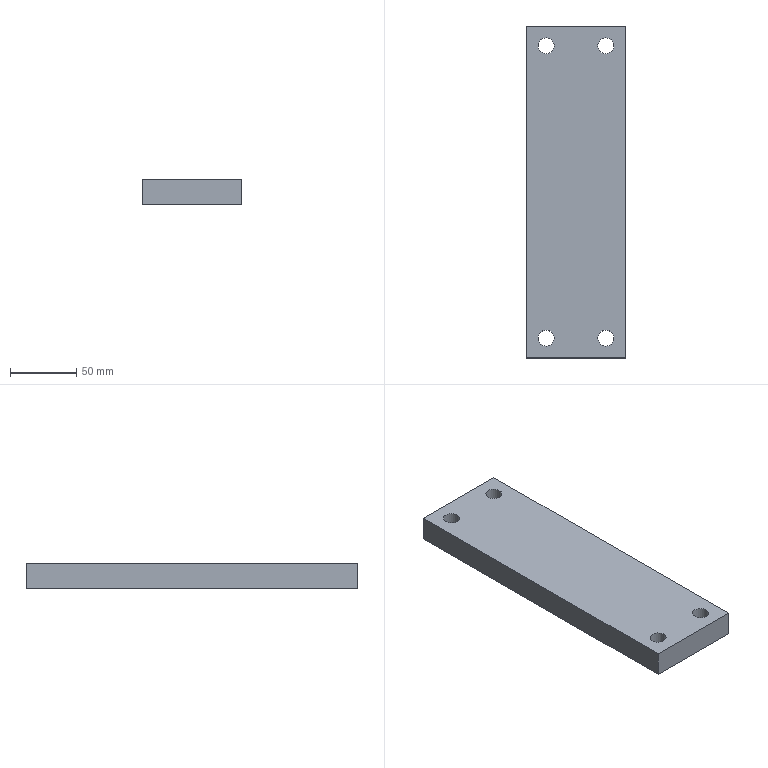Part | NX | features solid 2 | 1 solid | 10 faces | box 75 x 250 x 19 mm | volume 347655 mm3 | plane 6 | cylinder 4 | commonest cylinder face diameters 12 x4
STEP:
#1=CARTESIAN_POINT('',(277.5,-114.,-15.));
#2=VERTEX_POINT('',#1);
#3=CARTESIAN_POINT('',(277.5,-120.,-15.));
#4=DIRECTION('',(0.,0.,1.));
#5=DIRECTION('',(0.,1.,0.));
#6=AXIS2_PLACEMENT_3D('',#3,#4,#5);
#7=CIRCLE('',#6,6.);
#8=EDGE_CURVE('',#2,#2,#7,.T.);
#9=ORIENTED_EDGE('',*,*,#8,.F.);
#10=EDGE_LOOP('',(#9));
#11=FACE_BOUND('',#10,.T.);
#12=CARTESIAN_POINT('',(277.5,106.,-15.));
#13=VERTEX_POINT('',#12);
#14=CARTESIAN_POINT('',(277.5,100.,-15.));
#15=DIRECTION('',(0.,0.,1.));
#16=DIRECTION('',(0.,1.,0.));
#17=AXIS2_PLACEMENT_3D('',#14,#15,#16);
#18=CIRCLE('',#17,6.);
#19=EDGE_CURVE('',#13,#13,#18,.F.);
#20=ORIENTED_EDGE('',*,*,#19,.T.);
#21=EDGE_LOOP('',(#20));
#22=FACE_BOUND('',#21,.T.);
#23=CARTESIAN_POINT('',(232.5,106.,-15.));
#24=VERTEX_POINT('',#23);
#25=CARTESIAN_POINT('',(232.5,100.,-15.));
#26=DIRECTION('',(0.,0.,1.));
#27=DIRECTION('',(0.,1.,0.));
#28=AXIS2_PLACEMENT_3D('',#25,#26,#27);
#29=CIRCLE('',#28,6.);
#30=EDGE_CURVE('',#24,#24,#29,.T.);
#31=ORIENTED_EDGE('',*,*,#30,.F.);
#32=EDGE_LOOP('',(#31));
#33=FACE_BOUND('',#32,.T.);
#34=CARTESIAN_POINT('',(292.5,115.,-15.));
#35=VERTEX_POINT('',#34);
#36=CARTESIAN_POINT('',(292.5,-135.,-15.));
#37=VERTEX_POINT('',#36);
#38=CARTESIAN_POINT('',(292.5,115.,-15.));
#39=DIRECTION('',(0.,-1.,0.));
#40=VECTOR('',#39,1000.);
#41=LINE('',#38,#40);
#42=EDGE_CURVE('',#35,#37,#41,.T.);
#43=ORIENTED_EDGE('',*,*,#42,.F.);
#44=CARTESIAN_POINT('',(217.5,115.,-15.));
#45=VERTEX_POINT('',#44);
#46=CARTESIAN_POINT('',(217.5,115.,-15.));
#47=DIRECTION('',(1.,0.,0.));
#48=VECTOR('',#47,1000.);
#49=LINE('',#46,#48);
#50=EDGE_CURVE('',#45,#35,#49,.T.);
#51=ORIENTED_EDGE('',*,*,#50,.F.);
#52=CARTESIAN_POINT('',(217.5,-135.,-15.));
#53=VERTEX_POINT('',#52);
#54=CARTESIAN_POINT('',(217.5,-135.,-15.));
#55=DIRECTION('',(0.,1.,0.));
#56=VECTOR('',#55,1000.);
#57=LINE('',#54,#56);
#58=EDGE_CURVE('',#53,#45,#57,.T.);
#59=ORIENTED_EDGE('',*,*,#58,.F.);
#60=CARTESIAN_POINT('',(292.5,-135.,-15.));
#61=DIRECTION('',(-1.,0.,0.));
#62=VECTOR('',#61,1000.);
#63=LINE('',#60,#62);
#64=EDGE_CURVE('',#37,#53,#63,.T.);
#65=ORIENTED_EDGE('',*,*,#64,.F.);
#66=EDGE_LOOP('',(#43,#51,#59,#65));
#67=FACE_BOUND('',#66,.T.);
#68=CARTESIAN_POINT('',(232.5,-114.,-15.));
#69=VERTEX_POINT('',#68);
#70=CARTESIAN_POINT('',(232.5,-120.,-15.));
#71=DIRECTION('',(0.,0.,1.));
#72=DIRECTION('',(0.,1.,0.));
#73=AXIS2_PLACEMENT_3D('',#70,#71,#72);
#74=CIRCLE('',#73,6.);
#75=EDGE_CURVE('',#69,#69,#74,.F.);
#76=ORIENTED_EDGE('',*,*,#75,.T.);
#77=EDGE_LOOP('',(#76));
#78=FACE_BOUND('',#77,.T.);
#79=CARTESIAN_POINT('',(292.5,115.,-15.));
#80=DIRECTION('',(0.,0.,1.));
#81=DIRECTION('',(0.,1.,0.));
#82=AXIS2_PLACEMENT_3D('',#79,#80,#81);
#83=PLANE('',#82);
#84=ADVANCED_FACE('',(#11,#22,#33,#67,#78),#83,.T.);
#85=CARTESIAN_POINT('',(277.5,-114.,-34.));
#86=VERTEX_POINT('',#85);
#87=CARTESIAN_POINT('',(277.5,-120.,-34.));
#88=DIRECTION('',(0.,0.,1.));
#89=DIRECTION('',(0.,1.,0.));
#90=AXIS2_PLACEMENT_3D('',#87,#88,#89);
#91=CIRCLE('',#90,6.);
#92=EDGE_CURVE('',#86,#86,#91,.T.);
#93=ORIENTED_EDGE('',*,*,#92,.T.);
#94=EDGE_LOOP('',(#93));
#95=FACE_BOUND('',#94,.T.);
#96=CARTESIAN_POINT('',(277.5,106.,-34.));
#97=VERTEX_POINT('',#96);
#98=CARTESIAN_POINT('',(277.5,100.,-34.));
#99=DIRECTION('',(0.,0.,1.));
#100=DIRECTION('',(0.,1.,0.));
#101=AXIS2_PLACEMENT_3D('',#98,#99,#100);
#102=CIRCLE('',#101,6.);
#103=EDGE_CURVE('',#97,#97,#102,.F.);
#104=ORIENTED_EDGE('',*,*,#103,.F.);
#105=EDGE_LOOP('',(#104));
#106=FACE_BOUND('',#105,.T.);
#107=CARTESIAN_POINT('',(232.5,106.,-34.));
#108=VERTEX_POINT('',#107);
#109=CARTESIAN_POINT('',(232.5,100.,-34.));
#110=DIRECTION('',(0.,0.,1.));
#111=DIRECTION('',(0.,1.,0.));
#112=AXIS2_PLACEMENT_3D('',#109,#110,#111);
#113=CIRCLE('',#112,6.);
#114=EDGE_CURVE('',#108,#108,#113,.T.);
#115=ORIENTED_EDGE('',*,*,#114,.T.);
#116=EDGE_LOOP('',(#115));
#117=FACE_BOUND('',#116,.T.);
#118=CARTESIAN_POINT('',(292.5,115.,-34.));
#119=VERTEX_POINT('',#118);
#120=CARTESIAN_POINT('',(292.5,-135.,-34.));
#121=VERTEX_POINT('',#120);
#122=CARTESIAN_POINT('',(292.5,115.,-34.));
#123=DIRECTION('',(0.,-1.,0.));
#124=VECTOR('',#123,1000.);
#125=LINE('',#122,#124);
#126=EDGE_CURVE('',#119,#121,#125,.T.);
#127=ORIENTED_EDGE('',*,*,#126,.T.);
#128=CARTESIAN_POINT('',(217.5,-135.,-34.));
#129=VERTEX_POINT('',#128);
#130=CARTESIAN_POINT('',(292.5,-135.,-34.));
#131=DIRECTION('',(-1.,0.,0.));
#132=VECTOR('',#131,1000.);
#133=LINE('',#130,#132);
#134=EDGE_CURVE('',#121,#129,#133,.T.);
#135=ORIENTED_EDGE('',*,*,#134,.T.);
#136=CARTESIAN_POINT('',(217.5,115.,-34.));
#137=VERTEX_POINT('',#136);
#138=CARTESIAN_POINT('',(217.5,-135.,-34.));
#139=DIRECTION('',(0.,1.,0.));
#140=VECTOR('',#139,1000.);
#141=LINE('',#138,#140);
#142=EDGE_CURVE('',#129,#137,#141,.T.);
#143=ORIENTED_EDGE('',*,*,#142,.T.);
#144=CARTESIAN_POINT('',(217.5,115.,-34.));
#145=DIRECTION('',(1.,0.,0.));
#146=VECTOR('',#145,1000.);
#147=LINE('',#144,#146);
#148=EDGE_CURVE('',#137,#119,#147,.T.);
#149=ORIENTED_EDGE('',*,*,#148,.T.);
#150=EDGE_LOOP('',(#127,#135,#143,#149));
#151=FACE_BOUND('',#150,.T.);
#152=CARTESIAN_POINT('',(232.5,-114.,-34.));
#153=VERTEX_POINT('',#152);
#154=CARTESIAN_POINT('',(232.5,-120.,-34.));
#155=DIRECTION('',(0.,0.,1.));
#156=DIRECTION('',(0.,1.,0.));
#157=AXIS2_PLACEMENT_3D('',#154,#155,#156);
#158=CIRCLE('',#157,6.);
#159=EDGE_CURVE('',#153,#153,#158,.F.);
#160=ORIENTED_EDGE('',*,*,#159,.F.);
#161=EDGE_LOOP('',(#160));
#162=FACE_BOUND('',#161,.T.);
#163=CARTESIAN_POINT('',(292.5,115.,-34.));
#164=DIRECTION('',(0.,0.,1.));
#165=DIRECTION('',(0.,1.,0.));
#166=AXIS2_PLACEMENT_3D('',#163,#164,#165);
#167=PLANE('',#166);
#168=ADVANCED_FACE('',(#95,#106,#117,#151,#162),#167,.F.);
#169=ORIENTED_EDGE('',*,*,#126,.F.);
#170=CARTESIAN_POINT('',(292.5,115.,-15.));
#171=DIRECTION('',(0.,0.,-1.));
#172=VECTOR('',#171,1000.);
#173=LINE('',#170,#172);
#174=EDGE_CURVE('',#35,#119,#173,.T.);
#175=ORIENTED_EDGE('',*,*,#174,.F.);
#176=ORIENTED_EDGE('',*,*,#42,.T.);
#177=CARTESIAN_POINT('',(292.5,-135.,-15.));
#178=DIRECTION('',(0.,0.,-1.));
#179=VECTOR('',#178,1000.);
#180=LINE('',#177,#179);
#181=EDGE_CURVE('',#37,#121,#180,.T.);
#182=ORIENTED_EDGE('',*,*,#181,.T.);
#183=EDGE_LOOP('',(#169,#175,#176,#182));
#184=FACE_BOUND('',#183,.T.);
#185=CARTESIAN_POINT('',(292.5,115.,-15.));
#186=DIRECTION('',(1.,0.,0.));
#187=DIRECTION('',(0.,1.,0.));
#188=AXIS2_PLACEMENT_3D('',#185,#186,#187);
#189=PLANE('',#188);
#190=ADVANCED_FACE('',(#184),#189,.T.);
#191=ORIENTED_EDGE('',*,*,#134,.F.);
#192=ORIENTED_EDGE('',*,*,#181,.F.);
#193=ORIENTED_EDGE('',*,*,#64,.T.);
#194=CARTESIAN_POINT('',(217.5,-135.,-15.));
#195=DIRECTION('',(0.,0.,-1.));
#196=VECTOR('',#195,1000.);
#197=LINE('',#194,#196);
#198=EDGE_CURVE('',#53,#129,#197,.T.);
#199=ORIENTED_EDGE('',*,*,#198,.T.);
#200=EDGE_LOOP('',(#191,#192,#193,#199));
#201=FACE_BOUND('',#200,.T.);
#202=CARTESIAN_POINT('',(292.5,-135.,-15.));
#203=DIRECTION('',(0.,-1.,0.));
#204=DIRECTION('',(1.,0.,0.));
#205=AXIS2_PLACEMENT_3D('',#202,#203,#204);
#206=PLANE('',#205);
#207=ADVANCED_FACE('',(#201),#206,.T.);
#208=ORIENTED_EDGE('',*,*,#142,.F.);
#209=ORIENTED_EDGE('',*,*,#198,.F.);
#210=ORIENTED_EDGE('',*,*,#58,.T.);
#211=CARTESIAN_POINT('',(217.5,115.,-15.));
#212=DIRECTION('',(0.,0.,-1.));
#213=VECTOR('',#212,1000.);
#214=LINE('',#211,#213);
#215=EDGE_CURVE('',#45,#137,#214,.T.);
#216=ORIENTED_EDGE('',*,*,#215,.T.);
#217=EDGE_LOOP('',(#208,#209,#210,#216));
#218=FACE_BOUND('',#217,.T.);
#219=CARTESIAN_POINT('',(217.5,-135.,-15.));
#220=DIRECTION('',(-1.,0.,0.));
#221=DIRECTION('',(0.,0.,1.));
#222=AXIS2_PLACEMENT_3D('',#219,#220,#221);
#223=PLANE('',#222);
#224=ADVANCED_FACE('',(#218),#223,.T.);
#225=ORIENTED_EDGE('',*,*,#148,.F.);
#226=ORIENTED_EDGE('',*,*,#215,.F.);
#227=ORIENTED_EDGE('',*,*,#50,.T.);
#228=ORIENTED_EDGE('',*,*,#174,.T.);
#229=EDGE_LOOP('',(#225,#226,#227,#228));
#230=FACE_BOUND('',#229,.T.);
#231=CARTESIAN_POINT('',(217.5,115.,-15.));
#232=DIRECTION('',(0.,1.,0.));
#233=DIRECTION('',(0.,0.,-1.));
#234=AXIS2_PLACEMENT_3D('',#231,#232,#233);
#235=PLANE('',#234);
#236=ADVANCED_FACE('',(#230),#235,.T.);
#237=ORIENTED_EDGE('',*,*,#30,.T.);
#238=EDGE_LOOP('',(#237));
#239=FACE_BOUND('',#238,.T.);
#240=ORIENTED_EDGE('',*,*,#114,.F.);
#241=EDGE_LOOP('',(#240));
#242=FACE_BOUND('',#241,.T.);
#243=CARTESIAN_POINT('',(232.5,100.,-220.));
#244=DIRECTION('',(0.,0.,1.));
#245=DIRECTION('',(0.,1.,0.));
#246=AXIS2_PLACEMENT_3D('',#243,#244,#245);
#247=CYLINDRICAL_SURFACE('',#246,6.);
#248=ADVANCED_FACE('',(#239,#242),#247,.F.);
#249=ORIENTED_EDGE('',*,*,#19,.F.);
#250=EDGE_LOOP('',(#249));
#251=FACE_BOUND('',#250,.T.);
#252=ORIENTED_EDGE('',*,*,#103,.T.);
#253=EDGE_LOOP('',(#252));
#254=FACE_BOUND('',#253,.T.);
#255=CARTESIAN_POINT('',(277.5,100.,-220.));
#256=DIRECTION('',(0.,0.,1.));
#257=DIRECTION('',(0.,1.,0.));
#258=AXIS2_PLACEMENT_3D('',#255,#256,#257);
#259=CYLINDRICAL_SURFACE('',#258,6.);
#260=ADVANCED_FACE('',(#251,#254),#259,.F.);
#261=ORIENTED_EDGE('',*,*,#75,.F.);
#262=EDGE_LOOP('',(#261));
#263=FACE_BOUND('',#262,.T.);
#264=ORIENTED_EDGE('',*,*,#159,.T.);
#265=EDGE_LOOP('',(#264));
#266=FACE_BOUND('',#265,.T.);
#267=CARTESIAN_POINT('',(232.5,-120.,-220.));
#268=DIRECTION('',(0.,0.,1.));
#269=DIRECTION('',(0.,1.,0.));
#270=AXIS2_PLACEMENT_3D('',#267,#268,#269);
#271=CYLINDRICAL_SURFACE('',#270,6.);
#272=ADVANCED_FACE('',(#263,#266),#271,.F.);
#273=ORIENTED_EDGE('',*,*,#8,.T.);
#274=EDGE_LOOP('',(#273));
#275=FACE_BOUND('',#274,.T.);
#276=ORIENTED_EDGE('',*,*,#92,.F.);
#277=EDGE_LOOP('',(#276));
#278=FACE_BOUND('',#277,.T.);
#279=CARTESIAN_POINT('',(277.5,-120.,-220.));
#280=DIRECTION('',(0.,0.,1.));
#281=DIRECTION('',(0.,1.,0.));
#282=AXIS2_PLACEMENT_3D('',#279,#280,#281);
#283=CYLINDRICAL_SURFACE('',#282,6.);
#284=ADVANCED_FACE('',(#275,#278),#283,.F.);
#285=CLOSED_SHELL('',(#84,#168,#190,#207,#224,#236,#248,#260,#272,#284));
#286=MANIFOLD_SOLID_BREP('',#285);
#287=(LENGTH_UNIT()NAMED_UNIT(*)SI_UNIT(.MILLI.,.METRE.));
#288=UNCERTAINTY_MEASURE_WITH_UNIT(LENGTH_MEASURE(0.00001),#287,'','');
#289=(NAMED_UNIT(*)PLANE_ANGLE_UNIT()SI_UNIT($,.RADIAN.));
#290=(NAMED_UNIT(*)SI_UNIT($,.STERADIAN.)SOLID_ANGLE_UNIT());
#291=(GEOMETRIC_REPRESENTATION_CONTEXT(3)GLOBAL_UNCERTAINTY_ASSIGNED_CONTEXT((#288))GLOBAL_UNIT_ASSIGNED_CONTEXT((#287,#289,#290))REPRESENTATION_CONTEXT('',''));
#292=ADVANCED_BREP_SHAPE_REPRESENTATION('',(#286),#291);